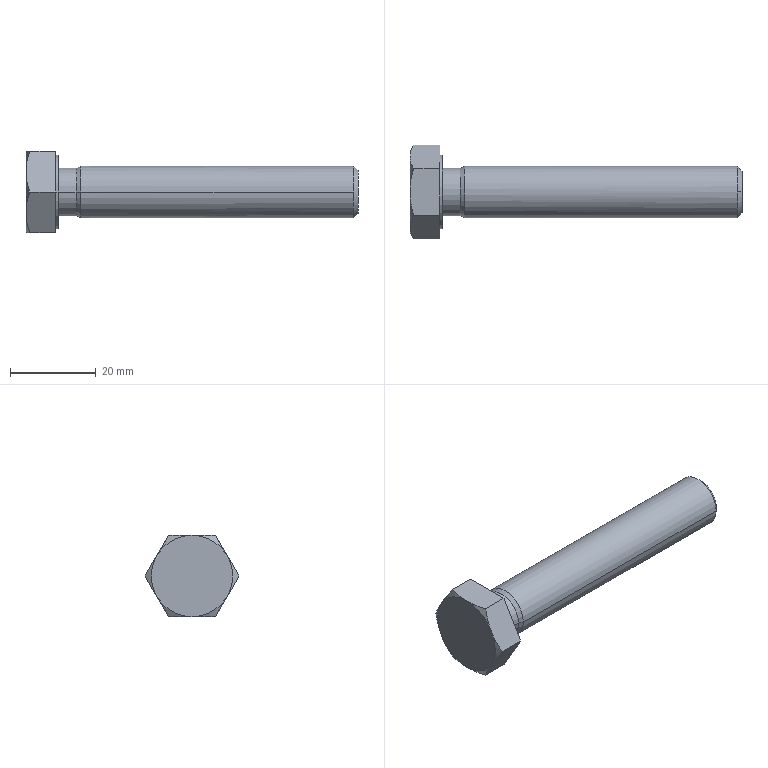Part | STEP file | DIN 933 - M12  x 70 | 1 solid | 26 faces | box 77.5 x 21.939 x 19 mm | volume 10105 mm3 | cone 10 | plane 10 | cylinder 6 | commonest cylinder face diameters 11.053 x2 12 x2 17.2 x2